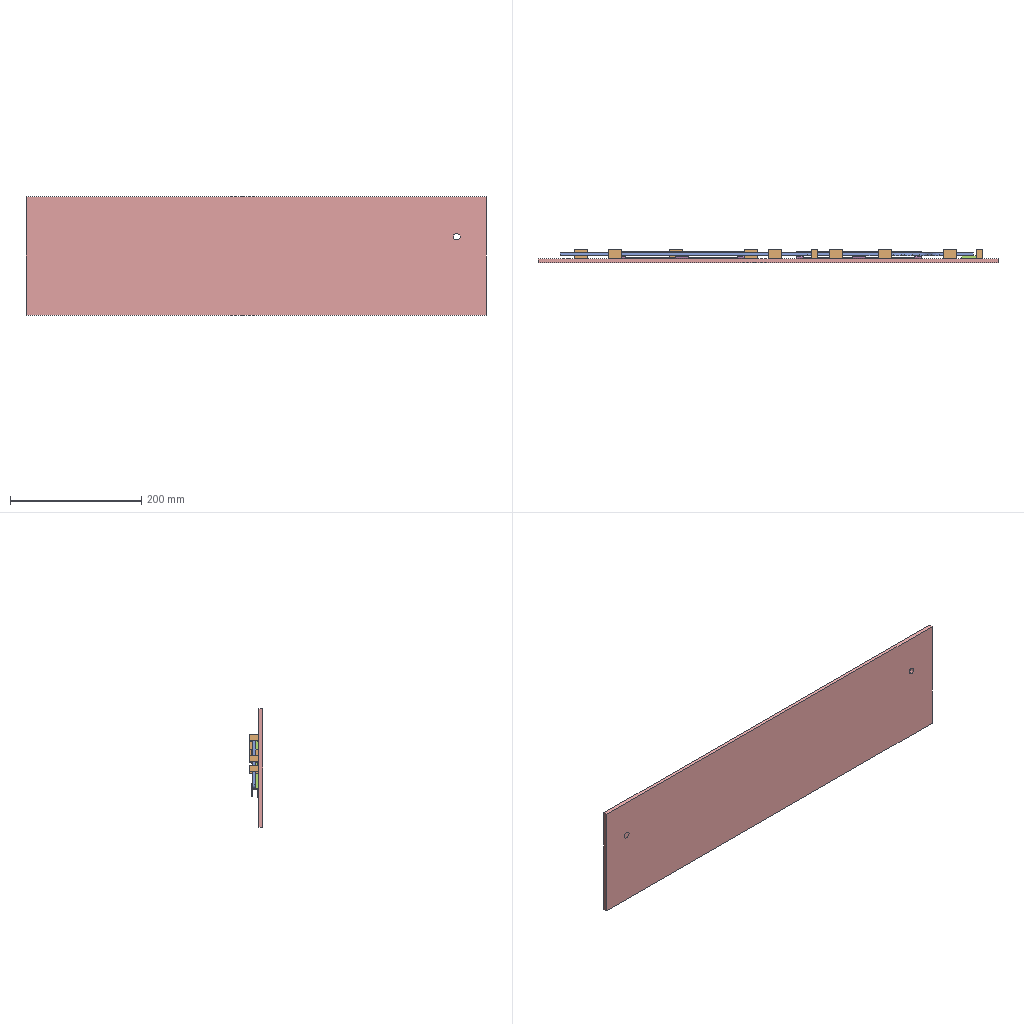Assembly | SolidWorks | 7 different items | 18 placed | box 700 x 21 x 180 mm
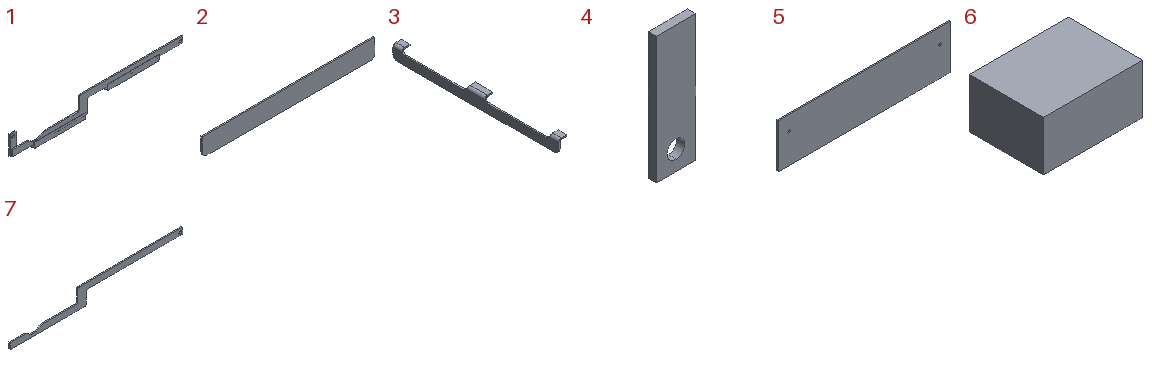Parts list (item | name | quantity | parent item | size | volume | features):
1 | (subassembly) | x1 | - | 633.1 x 11.2 x 87 mm | 92876 mm3 | -
2 | - | x2 | in 1 | 190 x 1.6 x 20 mm | 6063 mm3 | features Extrusion 1
3 | - | x2 | in 1 | 9.6 x 190 x 15 mm | 3822 mm3 | features ICE 2, FlatPattern 1, SMBaseFlange 1, SheetMetal 1
4 | - | x1 | in 1 | 22 x 4.5 x 71 mm | 6676 mm3 | features Extrusion 1
5 | - | x1 | - | 700 x 6 x 180 mm | 755105 mm3 | features Cut 2, FlatPattern 1, SMBaseFlange 1, SheetMetal 1
6 | - | x10 | - | 20 x 15 x 10 mm | 3000 mm3 | features Extrusion 1
7 | - | x1 | in 1 | 628.5 x 4.5 x 72 mm | 66431 mm3 | features Extrusion 1
Mates (type | each side: item.copy, entity, surface, feature):
In the top assembly
Coincident | 5.1 face plane Base-Flange1 | 6.1 face plane Boss-Extrude1
Coincident | 6.2 face plane Boss-Extrude1 | 6.3 face plane Boss-Extrude1
Coincident | 6.1 face plane Boss-Extrude1 | 6.4 face plane Boss-Extrude1
Coincident | 6.5 face plane Boss-Extrude1 | 6.6 face plane Boss-Extrude1
Coincident | 6.7 face plane Boss-Extrude1 | 6.5 face plane Boss-Extrude1
Coincident | 6.4 face plane Boss-Extrude1 | 6.5 face plane Boss-Extrude1
Coincident | 6.8 face plane Boss-Extrude1 | 6.9 face plane Boss-Extrude1
Coincident | 6.8 face plane Boss-Extrude1 | 6.10 face plane Boss-Extrude1
Coincident | 6.7 face plane Boss-Extrude1 | 6.9 face plane Boss-Extrude1
Coincident | 4.1 face plane Boss-Extrude1 | 6.9 face plane Boss-Extrude1
Coincident | 7.1 face plane Boss-Extrude1 | 6.7 face plane Boss-Extrude1
DistanceDim | 7.1 face plane Boss-Extrude1 | 5.1 face plane Base-Flange1
DistanceDim | 3.1 face plane Base-Flange1 | 5.1 face plane Base-Flange1
Coincident | 5.1 face plane Base-Flange1 | 3.1 face plane Base-Flange1
Coincident | 7.1 face plane Boss-Extrude1 | 6.4 face plane Boss-Extrude1
Coincident | 7.1 face plane Boss-Extrude1 | 6.1 face plane Boss-Extrude1
Coincident | 3.2 face plane Base-Flange1 | 6.5 face plane Boss-Extrude1
Coincident | 3.2 face plane Base-Flange1 | 6.10 face plane Boss-Extrude1
Coincident | 7.1 face plane Boss-Extrude1 | 6.10 face plane Boss-Extrude1
Coincident | 7.1 face plane Boss-Extrude1 | 6.8 face plane Boss-Extrude1
Coincident | 5.1 face plane Base-Flange1 | 6.2 face plane Boss-Extrude1
Coincident | 7.1 face plane Boss-Extrude1 | 6.2 face plane Boss-Extrude1
Coincident | 7.1 face plane Boss-Extrude1 | 6.6 face plane Boss-Extrude1
Coincident | 7.1 face plane Boss-Extrude1 | 6.3 face plane Boss-Extrude1
In subassembly 1
Coincident | 7.2 face plane Boss-Extrude1 | 4.2 face plane Boss-Extrude1 | 2 times
DistanceDim | 4.2 face plane Boss-Extrude1 | 7.2 face plane Boss-Extrude1
Coincident | 3.3 face plane Base-Flange1 | 2.1 face plane Boss-Extrude1 | 2 times
DistanceDim | 3.3 face plane Base-Flange1 | 2.1 face plane Boss-Extrude1
Coincident | 7.2 face plane Boss-Extrude1 | 3.3 face plane Base-Flange1
Coincident | 7.2 face plane Boss-Extrude1 | 2.1 face plane Boss-Extrude1
DistanceDim | 2.1 face plane Boss-Extrude1 | 7.2 face plane Boss-Extrude1
Coincident | 2.2 face plane Boss-Extrude1 | 3.4 face plane Base-Flange1 | 2 times
DistanceDim | 3.4 face plane Base-Flange1 | 2.2 face plane Boss-Extrude1
Coincident | 7.2 face plane Boss-Extrude1 | 2.2 face plane Boss-Extrude1
Coincident | 7.2 face plane Boss-Extrude1 | 3.4 face plane Base-Flange1
DistanceDim | 3.4 face plane Base-Flange1 | 7.2 face plane Boss-Extrude1